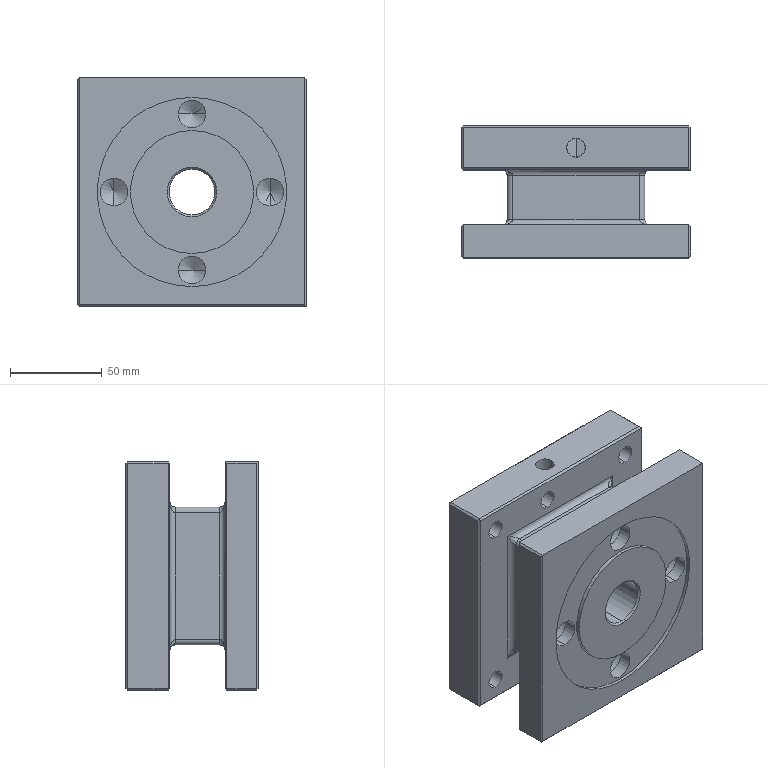Part | SolidWorks | features ICE 7, Fillet 2, HoleWzd 2, Chamfer 1, CirPattern 1, Extrusion 1, RevCut 1 | 1 solid | 121 faces | box 125 x 72 x 125 mm | volume 738027 mm3 | plane 49 | cylinder 46 | cone 18 | spline 8 | commonest cylinder face diameters 10.2 x14 6 x12 15 x8 10 x2 25 x2 36 x2